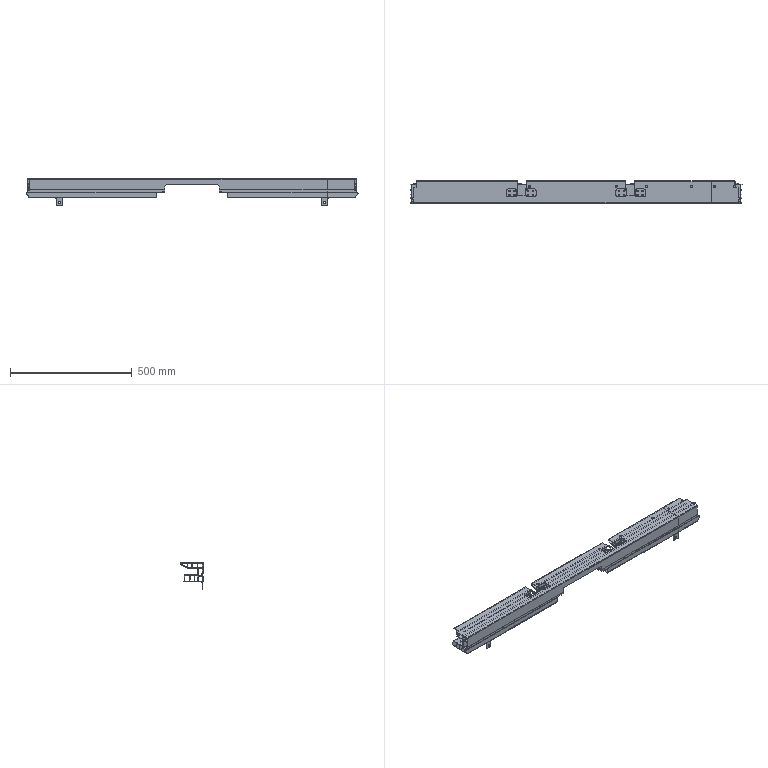NC program | NX | posted with a generic post | part box 1365 x 90.95 x 108.501 mm
Lines 22022 to 22311 of 22311:
(ZLEVEL_PROFILE_COPY_1_COPY_COPY_COPY_COPY , TOOL : D6A45)
N43958 T07 M6
N43960 G54
N43962 G17 G0 G90 X-421.753 Y2.707 B0. C0. S6000 M3
N43964 G43 Z30. H7
N43966 Z-31.
N43968 G94 G1 X-422.48 Y3.966 F1000.
N43970 G3 X-423. Y4.266 R0.6
N43972 X-426.541 Y0.725 R3.541
N43974 X-423. Y4.266 R-3.541
N43976 X-423.52 Y3.966 R0.6
N43978 G1 X-424.247 Y2.707
N43980 G0 Z30.
N43982 X-371.753
N43984 Z-31.
N43986 G1 X-372.48 Y3.966
N43988 G3 X-373. Y4.266 R0.6
N43990 X-376.541 Y0.725 R3.541
N43992 X-373. Y4.266 R-3.541
N43994 X-373.52 Y3.966 R0.6
N43996 G1 X-374.247 Y2.707
N43998 G0 Z30.
N44000 X-326.753
N44002 Z-31.
N44004 G1 X-327.48 Y3.966
N44006 G3 X-328. Y4.266 R0.6
N44008 X-331.541 Y0.725 R3.541
N44010 X-328. Y4.266 R-3.541
N44012 X-328.52 Y3.966 R0.6
N44014 G1 X-329.247 Y2.707
N44016 G0 Z30.
N44018 X-276.753
N44020 Z-31.
N44022 G1 X-277.48 Y3.966
N44024 G3 X-278. Y4.266 R0.6
N44026 X-281.541 Y0.725 R3.541
N44028 X-278. Y4.266 R-3.541
N44030 X-278.52 Y3.966 R0.6
N44032 G1 X-279.247 Y2.707
N44034 G0 Z30.
N44036 X-246.753
N44038 Z-31.
N44040 G1 X-247.48 Y3.966
N44042 G3 X-248. Y4.266 R0.6
N44044 G1 X-248.004
N44046 G3 X-251.541 Y0.721 R3.541
N44048 X-248. Y4.266 R-3.541
N44050 X-248.52 Y3.966 R0.6
N44052 G1 X-249.247 Y2.707
N44054 G0 Z30.
N44056 X-601.054 Y-21.141
N44058 Z-31.
N44060 G1 X-600.52 Y-22.067
N44062 G3 X-600. Y-22.367 R0.6
N44064 X-577.459 Y0.175 R22.541
N44066 X-600. Y-22.367 R-22.541
N44068 X-599.48 Y-22.067 R0.6
N44070 G1 X-598.946 Y-21.141
N44072 G0 Z30.
N44074 X-365.983 Y-20.507
N44076 Z-31.
N44078 G1 X-365.256 Y-21.766
N44080 G3 X-364.736 Y-22.066 R0.6
N44082 X-361.195 Y-18.525 R3.541
N44084 X-364.736 Y-22.066 R-3.541
N44086 X-364.216 Y-21.766 R0.6
N44088 G1 X-363.489 Y-20.507
N44090 G0 Z30.
N44092 X-315.983
N44094 Z-31.
N44096 G1 X-315.256 Y-21.766
N44098 G3 X-314.736 Y-22.066 R0.6
N44100 X-311.194 Y-18.525 R3.541
N44102 X-314.736 Y-22.066 R-3.541
N44104 X-314.216 Y-21.766 R0.6
N44106 G1 X-313.489 Y-20.507
N44108 G0 Z30.
N44110 X-265.983
N44112 Z-31.
N44114 G1 X-265.256 Y-21.766
N44116 G3 X-264.736 Y-22.066 R0.6
N44118 X-261.194 Y-18.525 R3.541
N44120 X-264.736 Y-22.066 R-3.541
N44122 X-264.216 Y-21.766 R0.6
N44124 G1 X-263.489 Y-20.507
N44126 G0 Z30.
N44128 X-563.804 Y-1.532
N44130 Z-31.
N44132 G1 X-564.021 Y-2.466
N44134 G3 X-563.501 Y-2.766 R0.6
N44136 X-560.96 Y-0.225 R2.541
N44138 X-563.501 Y-2.766 R-2.541
N44140 X-562.981 Y-2.466 R0.6
N44142 G1 X-563.198 Y-1.532
N44144 G0 Z30.
N44146 X-636.803 Y-1.132
N44148 Z-31.
N44150 G1 X-637.02 Y-2.066
N44152 G3 X-636.5 Y-2.366 R0.6
N44154 X-633.959 Y0.175 R2.541
N44156 X-636.5 Y-2.366 R-2.541
N44158 X-635.98 Y-2.066 R0.6
N44160 G1 X-636.197 Y-1.132
N44162 G0 Z30.
N44164 X249.247 Y2.707
N44166 Z-31.
N44168 G1 X248.52 Y3.966
N44170 G3 X248. Y4.266 R0.6
N44172 X244.459 Y0.725 R3.541
N44174 X248. Y4.266 R-3.541
N44176 X247.48 Y3.966 R0.6
N44178 G1 X246.753 Y2.707
N44180 G0 Z30.
N44182 X279.247
N44184 Z-31.
N44186 G1 X278.52 Y3.966
N44188 G3 X278. Y4.266 R0.6
N44190 X274.459 Y0.725 R3.541
N44192 X278. Y4.266 R-3.541
N44194 X277.48 Y3.966 R0.6
N44196 G1 X276.753 Y2.707
N44198 G0 Z30.
N44200 X329.247
N44202 Z-31.
N44204 G1 X328.52 Y3.966
N44206 G3 X328. Y4.266 R0.6
N44208 X324.459 Y0.725 R3.541
N44210 X328. Y4.266 R-3.541
N44212 X327.48 Y3.966 R0.6
N44214 G1 X326.753 Y2.707
N44216 G0 Z30.
N44218 X374.247
N44220 Z-31.
N44222 G1 X373.52 Y3.966
N44224 G3 X373. Y4.266 R0.6
N44226 X369.459 Y0.725 R3.541
N44228 X373. Y4.266 R-3.541
N44230 X372.48 Y3.966 R0.6
N44232 G1 X371.753 Y2.707
N44234 G0 Z30.
N44236 X424.247
N44238 Z-31.
N44240 G1 X423.52 Y3.966
N44242 G3 X423. Y4.266 R0.6
N44244 X419.459 Y0.725 R3.541
N44246 X423. Y4.266 R-3.541
N44248 X422.48 Y3.966 R0.6
N44250 G1 X421.753 Y2.707
N44252 G0 Z30.
N44254 X598.946 Y-21.141
N44256 Z-31.
N44258 G1 X599.48 Y-22.067
N44260 G3 X600. Y-22.367 R0.6
N44262 X622.541 Y0.175 R22.541
N44264 X600. Y-22.367 R-22.541
N44266 X600.52 Y-22.067 R0.6
N44268 G1 X601.054 Y-21.141
N44270 G0 Z30.
N44272 X263.489 Y-20.507
N44274 Z-31.
N44276 G1 X264.216 Y-21.766
N44278 G3 X264.736 Y-22.066 R0.6
N44280 X268.277 Y-18.525 R3.541
N44282 X264.736 Y-22.066 R-3.541
N44284 X265.256 Y-21.766 R0.6
N44286 G1 X265.983 Y-20.507
N44288 G0 Z30.
N44290 X313.489
N44292 Z-31.
N44294 G1 X314.216 Y-21.766
N44296 G3 X314.736 Y-22.066 R0.6
N44298 X318.277 Y-18.525 R3.541
N44300 X314.736 Y-22.066 R-3.541
N44302 X315.256 Y-21.766 R0.6
N44304 G1 X315.983 Y-20.507
N44306 G0 Z30.
N44308 X363.489
N44310 Z-31.
N44312 G1 X364.216 Y-21.766
N44314 G3 X364.736 Y-22.066 R0.6
N44316 X368.277 Y-18.525 R3.541
N44318 X364.736 Y-22.066 R-3.541
N44320 X365.256 Y-21.766 R0.6
N44322 G1 X365.983 Y-20.507
N44324 G0 Z30.
N44326 X636.196 Y-1.532
N44328 Z-31.
N44330 G1 X635.979 Y-2.466
N44332 G3 X636.499 Y-2.766 R0.6
N44334 X639.04 Y-0.225 R2.541
N44336 X636.499 Y-2.766 R-2.541
N44338 X637.019 Y-2.466 R0.6
N44340 G1 X636.802 Y-1.532
N44342 G0 Z30.
N44344 X563.197 Y-1.132
N44346 Z-31.
N44348 G1 X562.98 Y-2.066
N44350 G3 X563.5 Y-2.366 R0.6
N44352 X566.041 Y0.175 R2.541
N44354 X563.5 Y-2.366 R-2.541
N44356 X564.02 Y-2.066 R0.6
N44358 G1 X563.803 Y-1.132
N44360 G0 Z30.
N44362 X146.822 Y-36.964
N44364 Z-31.
N44366 G1 X147.218 Y-36.225
N44368 G3 X147.199 Y-35.625 R0.6
N44370 G1 X143.869 Y-32.294
N44372 G2 X143.588 Y-31.618 R0.956
N44374 G1 Y43.976
N44376 G2 X143.869 Y44.652 R0.957
N44378 G1 X145.129 Y45.913
N44380 G2 X145.833 Y46.193 R0.975
N44382 G1 X528.094 Y46.195
N44384 G3 X528.613 Y46.495 R0.6
N44386 G1 X528.42 Y47.408
N44388 G0 Z30.
N44390 X561.583
N44392 Z-31.
N44394 G1 X561.391 Y46.495
N44396 G3 X561.911 Y46.195 R0.6
N44398 G1 X667.931 Y46.193
N44400 G3 X668.141 Y46.408 R0.3
N44402 G1 X668.399 Y47.421
N44404 G0 Z30.
N44406 X-668.401
N44408 Z-31.
N44410 G1 X-668.142 Y46.408
N44412 G3 X-667.932 Y46.193 R0.3
N44414 G1 X-561.905 Y46.195
N44416 G3 X-561.386 Y46.495 R0.6
N44418 G1 X-561.58 Y47.408
N44420 G0 Z30.
N44422 X-528.418
N44424 Z-31.
N44426 G1 X-528.613 Y46.495
N44428 G3 X-528.094 Y46.195 R0.6
N44430 G1 X-145.833 Y46.193
N44432 G2 X-145.128 Y45.913 R0.976
N44434 G1 X-143.867 Y44.652
N44436 G2 X-143.587 Y43.976 R0.957
N44438 G1 Y-31.618
N44440 G2 X-143.867 Y-32.294 R0.956
N44442 G1 X-147.198 Y-35.625
N44444 G3 X-147.216 Y-36.225 R0.6
N44446 G1 X-146.82 Y-36.964
N44448 G0 Z30.
N44450 M5
(TOOL16 , TOOL : D16)
N44452 T16 M6
N44454 G54
N44456 G17 G0 G90 X-600. Y0.175 B0. C0. S6000 M3
N44458 G43 Z30. H16
N44460 Z-29.2
N44462 G41 G94 G1 X-587.914 Y-2.975 F1200. D16
N44464 G3 X-584.5 Y0.175 R3.16
N44466 X-584.5 Y0.175 Z-34.2 I-15.5 J0.
N44468 X-584.5 Y0.175 Z-39.2 I-15.5 J0.
N44470 X-584.5 Y0.175 Z-44.2 I-15.5 J0.
N44472 X-584.5 Y0.175 Z-49.2 I-15.5 J0.
N44474 X-584.5 Y0.175 Z-54.2 I-15.5 J0.
N44476 X-599.027 Y-15.295 Z-58. R-15.5
N44478 X-584.531 Y1.148 R15.5
N44480 X-599.027 Y-15.295 R-15.5
N44482 X-596.098 Y-11.69 R3.16
N44484 G40
N44486 G1 X-600. Y0.175
N44488 G0 Z30.
N44490 X600.
N44492 Z-29.2
N44494 G41 G1 X612.086 Y-2.975
N44496 G3 X615.5 Y0.175 R3.16
N44498 X615.5 Y0.175 Z-34.2 I-15.5 J0.
N44500 X615.5 Y0.175 Z-39.2 I-15.5 J0.
N44502 X615.5 Y0.175 Z-44.2 I-15.5 J0.
N44504 X615.5 Y0.175 Z-49.2 I-15.5 J0.
N44506 X615.5 Y0.175 Z-54.2 I-15.5 J0.
N44508 X600.973 Y-15.295 Z-58. R-15.5
N44510 X615.469 Y1.148 R15.5
N44512 X600.973 Y-15.295 R-15.5
N44514 X603.902 Y-11.69 R3.16
N44516 G40
N44518 G1 X600. Y0.175
N44520 G0 Z30.
N44522 M5
N44524 M2